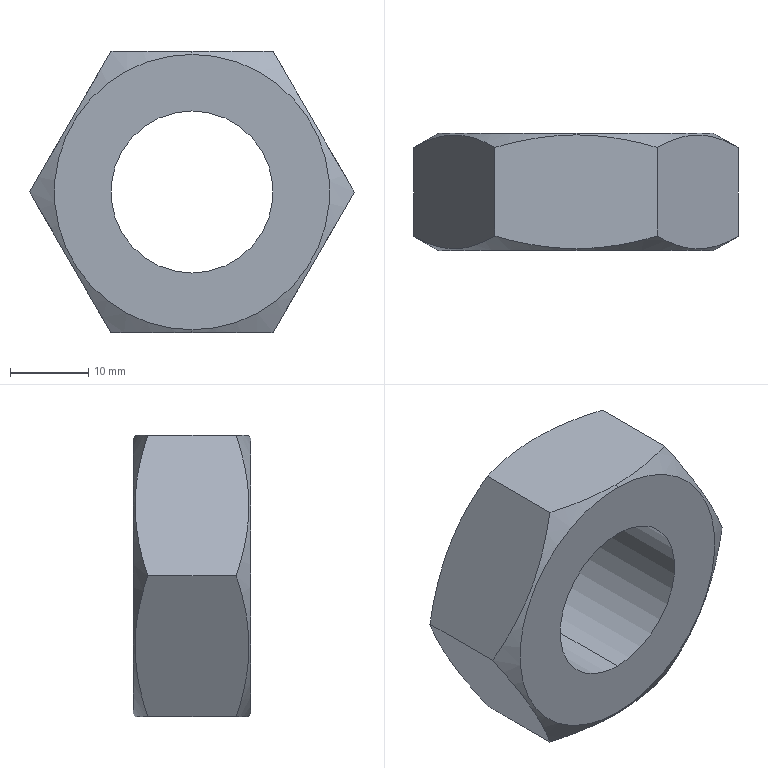Part | SolidWorks | features Extrusion 1, RevCut 1 | 1 solid | 14 faces | box 41.569 x 15 x 36.009 mm | volume 11607 mm3 | plane 8 | cone 4 | cylinder 2 | commonest cylinder face diameters 20.75 x2
STEP:
#1=CARTESIAN_POINT('',(0.,15.,-17.634));
#2=VERTEX_POINT('',#1);
#3=CARTESIAN_POINT('',(0.,15.,17.616));
#4=VERTEX_POINT('',#3);
#5=CARTESIAN_POINT('',(0.,15.,-0.008541));
#6=DIRECTION('',(0.,-1.,0.));
#7=DIRECTION('',(0.,0.,-1.));
#8=AXIS2_PLACEMENT_3D('',#5,#6,#7);
#9=CIRCLE('',#8,17.625);
#10=EDGE_CURVE('',#2,#4,#9,.T.);
#11=ORIENTED_EDGE('',*,*,#10,.T.);
#12=CARTESIAN_POINT('',(0.,14.779,18.));
#13=VERTEX_POINT('',#12);
#14=CARTESIAN_POINT('',(0.,14.786,17.987));
#15=DIRECTION('',(0.,-0.5,0.866));
#16=VECTOR('',#15,1000.);
#17=LINE('',#14,#16);
#18=EDGE_CURVE('',#4,#13,#17,.T.);
#19=ORIENTED_EDGE('',*,*,#18,.T.);
#20=CARTESIAN_POINT('',(10.4,13.172,17.996));
#21=VERTEX_POINT('',#20);
#22=CARTESIAN_POINT('',(10.4,13.172,17.996));
#23=CARTESIAN_POINT('',(8.698,13.662,17.996));
#24=CARTESIAN_POINT('',(6.985,14.067,17.997));
#25=CARTESIAN_POINT('',(3.522,14.626,17.999));
#26=CARTESIAN_POINT('',(1.772,14.779,17.999));
#27=CARTESIAN_POINT('',(0.,14.779,18.));
#28=B_SPLINE_CURVE_WITH_KNOTS('',3,(#22,#23,#24,#25,#26,#27),.UNSPECIFIED.,.F.,.F.,(4,2,4),(0.000000206,0.005261,0.01052),.UNSPECIFIED.);
#29=EDGE_CURVE('',#21,#13,#28,.T.);
#30=ORIENTED_EDGE('',*,*,#29,.F.);
#31=CARTESIAN_POINT('',(20.785,13.176,-0.008541));
#32=VERTEX_POINT('',#31);
#33=CARTESIAN_POINT('',(20.785,13.176,-0.008541));
#34=CARTESIAN_POINT('',(19.937,13.665,1.461));
#35=CARTESIAN_POINT('',(19.083,14.069,2.942));
#36=CARTESIAN_POINT('',(17.357,14.627,5.934));
#37=CARTESIAN_POINT('',(16.485,14.78,7.446));
#38=CARTESIAN_POINT('',(15.381,14.781,9.359));
#39=CARTESIAN_POINT('',(15.159,14.772,9.744));
#40=CARTESIAN_POINT('',(14.718,14.735,10.51));
#41=CARTESIAN_POINT('',(14.498,14.707,10.891));
#42=CARTESIAN_POINT('',(13.84,14.597,12.032));
#43=CARTESIAN_POINT('',(13.404,14.488,12.787));
#44=CARTESIAN_POINT('',(12.105,14.067,15.04));
#45=CARTESIAN_POINT('',(11.249,13.662,16.524));
#46=CARTESIAN_POINT('',(10.4,13.172,17.996));
#47=B_SPLINE_CURVE_WITH_KNOTS('',3,(#33,#34,#35,#36,#37,#38,#39,#40,#41,#42,#43,#44,#45,#46),.UNSPECIFIED.,.F.,.F.,(4,2,2,2,2,2,4),(0.000000238,0.005248,0.0105,0.01181,0.01312,0.01574,0.02099),.UNSPECIFIED.);
#48=EDGE_CURVE('',#32,#21,#47,.T.);
#49=ORIENTED_EDGE('',*,*,#48,.F.);
#50=CARTESIAN_POINT('',(10.385,13.18,-18.004));
#51=VERTEX_POINT('',#50);
#52=CARTESIAN_POINT('',(10.385,13.18,-18.004));
#53=CARTESIAN_POINT('',(11.234,13.67,-16.535));
#54=CARTESIAN_POINT('',(12.089,14.073,-15.055));
#55=CARTESIAN_POINT('',(13.818,14.632,-12.064));
#56=CARTESIAN_POINT('',(14.691,14.785,-10.553));
#57=CARTESIAN_POINT('',(15.796,14.786,-8.641));
#58=CARTESIAN_POINT('',(16.018,14.777,-8.256));
#59=CARTESIAN_POINT('',(16.461,14.74,-7.491));
#60=CARTESIAN_POINT('',(16.681,14.712,-7.11));
#61=CARTESIAN_POINT('',(17.34,14.602,-5.969));
#62=CARTESIAN_POINT('',(17.776,14.492,-5.214));
#63=CARTESIAN_POINT('',(19.077,14.072,-2.963));
#64=CARTESIAN_POINT('',(19.935,13.667,-1.479));
#65=CARTESIAN_POINT('',(20.785,13.176,-0.008541));
#66=B_SPLINE_CURVE_WITH_KNOTS('',3,(#52,#53,#54,#55,#56,#57,#58,#59,#60,#61,#62,#63,#64,#65),.UNSPECIFIED.,.F.,.F.,(4,2,2,2,2,2,4),(0.000000238,0.005248,0.0105,0.01181,0.01312,0.01574,0.02099),.UNSPECIFIED.);
#67=EDGE_CURVE('',#51,#32,#66,.T.);
#68=ORIENTED_EDGE('',*,*,#67,.F.);
#69=CARTESIAN_POINT('',(0.,14.788,-18.));
#70=VERTEX_POINT('',#69);
#71=CARTESIAN_POINT('',(0.,14.788,-18.));
#72=CARTESIAN_POINT('',(0.4407,14.788,-18.));
#73=CARTESIAN_POINT('',(0.8836,14.779,-18.));
#74=CARTESIAN_POINT('',(1.765,14.741,-18.001));
#75=CARTESIAN_POINT('',(2.204,14.713,-18.001));
#76=CARTESIAN_POINT('',(3.518,14.603,-18.001));
#77=CARTESIAN_POINT('',(4.388,14.494,-18.002));
#78=CARTESIAN_POINT('',(6.982,14.073,-18.003));
#79=CARTESIAN_POINT('',(8.69,13.669,-18.004));
#80=CARTESIAN_POINT('',(10.385,13.18,-18.004));
#81=B_SPLINE_CURVE_WITH_KNOTS('',3,(#71,#72,#73,#74,#75,#76,#77,#78,#79,#80),.UNSPECIFIED.,.F.,.F.,(4,2,2,2,4),(0.01052,0.01183,0.01314,0.01576,0.02099),.UNSPECIFIED.);
#82=EDGE_CURVE('',#70,#51,#81,.T.);
#83=ORIENTED_EDGE('',*,*,#82,.F.);
#84=CARTESIAN_POINT('',(0.,14.786,-18.004));
#85=DIRECTION('',(0.,-0.5,-0.866));
#86=VECTOR('',#85,1000.);
#87=LINE('',#84,#86);
#88=EDGE_CURVE('',#2,#70,#87,.T.);
#89=ORIENTED_EDGE('',*,*,#88,.F.);
#90=EDGE_LOOP('',(#11,#19,#30,#49,#68,#83,#89));
#91=FACE_OUTER_BOUND('',#90,.T.);
#92=CARTESIAN_POINT('',(0.,14.786,-0.008541));
#93=DIRECTION('',(0.,-1.,0.));
#94=DIRECTION('',(0.,0.,-1.));
#95=AXIS2_PLACEMENT_3D('',#92,#93,#94);
#96=CONICAL_SURFACE('',#95,17.996,1.047);
#97=ADVANCED_FACE('',(#91),#96,.T.);
#98=CARTESIAN_POINT('',(0.,0.,-17.634));
#99=VERTEX_POINT('',#98);
#100=CARTESIAN_POINT('',(0.,0.,17.616));
#101=VERTEX_POINT('',#100);
#102=CARTESIAN_POINT('',(0.,0.,-0.008541));
#103=DIRECTION('',(0.,-1.,0.));
#104=DIRECTION('',(0.,0.,-1.));
#105=AXIS2_PLACEMENT_3D('',#102,#103,#104);
#106=CIRCLE('',#105,17.625);
#107=EDGE_CURVE('',#99,#101,#106,.T.);
#108=ORIENTED_EDGE('',*,*,#107,.F.);
#109=CARTESIAN_POINT('',(0.,0.2116,-18.));
#110=VERTEX_POINT('',#109);
#111=CARTESIAN_POINT('',(0.,0.4553,-18.422));
#112=DIRECTION('',(0.,0.5,-0.866));
#113=VECTOR('',#112,1000.);
#114=LINE('',#111,#113);
#115=EDGE_CURVE('',#99,#110,#114,.T.);
#116=ORIENTED_EDGE('',*,*,#115,.T.);
#117=CARTESIAN_POINT('',(10.385,1.82,-18.004));
#118=VERTEX_POINT('',#117);
#119=CARTESIAN_POINT('',(10.385,1.82,-18.004));
#120=CARTESIAN_POINT('',(8.686,1.329,-18.004));
#121=CARTESIAN_POINT('',(6.975,0.9251,-18.003));
#122=CARTESIAN_POINT('',(3.517,0.3655,-18.001));
#123=CARTESIAN_POINT('',(1.769,0.212,-18.001));
#124=CARTESIAN_POINT('',(0.,0.2116,-18.));
#125=B_SPLINE_CURVE_WITH_KNOTS('',3,(#119,#120,#121,#122,#123,#124),.UNSPECIFIED.,.F.,.F.,(4,2,4),(0.000000206,0.005254,0.01051),.UNSPECIFIED.);
#126=EDGE_CURVE('',#118,#110,#125,.T.);
#127=ORIENTED_EDGE('',*,*,#126,.F.);
#128=CARTESIAN_POINT('',(20.785,1.824,-0.008541));
#129=VERTEX_POINT('',#128);
#130=CARTESIAN_POINT('',(20.785,1.824,-0.008541));
#131=CARTESIAN_POINT('',(19.936,1.334,-1.478));
#132=CARTESIAN_POINT('',(19.08,0.9299,-2.957));
#133=CARTESIAN_POINT('',(17.352,0.3698,-5.948));
#134=CARTESIAN_POINT('',(16.479,0.2156,-7.459));
#135=CARTESIAN_POINT('',(15.374,0.2137,-9.371));
#136=CARTESIAN_POINT('',(15.152,0.2227,-9.756));
#137=CARTESIAN_POINT('',(14.709,0.2595,-10.521));
#138=CARTESIAN_POINT('',(14.489,0.2872,-10.903));
#139=CARTESIAN_POINT('',(13.83,0.3968,-12.043));
#140=CARTESIAN_POINT('',(13.394,0.5054,-12.798));
#141=CARTESIAN_POINT('',(12.092,0.9251,-15.05));
#142=CARTESIAN_POINT('',(11.235,1.33,-16.533));
#143=CARTESIAN_POINT('',(10.385,1.82,-18.004));
#144=B_SPLINE_CURVE_WITH_KNOTS('',3,(#130,#131,#132,#133,#134,#135,#136,#137,#138,#139,#140,#141,#142,#143),.UNSPECIFIED.,.F.,.F.,(4,2,2,2,2,2,4),(0.000000238,0.005248,0.0105,0.01181,0.01312,0.01574,0.02099),.UNSPECIFIED.);
#145=EDGE_CURVE('',#129,#118,#144,.T.);
#146=ORIENTED_EDGE('',*,*,#145,.F.);
#147=CARTESIAN_POINT('',(10.4,1.828,17.996));
#148=VERTEX_POINT('',#147);
#149=CARTESIAN_POINT('',(10.4,1.828,17.996));
#150=CARTESIAN_POINT('',(11.247,1.338,16.526));
#151=CARTESIAN_POINT('',(12.101,0.9345,15.045));
#152=CARTESIAN_POINT('',(13.827,0.3746,12.053));
#153=CARTESIAN_POINT('',(14.699,0.2205,10.542));
#154=CARTESIAN_POINT('',(15.803,0.2186,8.628));
#155=CARTESIAN_POINT('',(16.025,0.2277,8.244));
#156=CARTESIAN_POINT('',(16.466,0.2644,7.478));
#157=CARTESIAN_POINT('',(16.686,0.2921,7.097));
#158=CARTESIAN_POINT('',(17.344,0.4016,5.956));
#159=CARTESIAN_POINT('',(17.78,0.5102,5.2));
#160=CARTESIAN_POINT('',(19.08,0.9297,2.947));
#161=CARTESIAN_POINT('',(19.936,1.334,1.463));
#162=CARTESIAN_POINT('',(20.785,1.824,-0.008541));
#163=B_SPLINE_CURVE_WITH_KNOTS('',3,(#149,#150,#151,#152,#153,#154,#155,#156,#157,#158,#159,#160,#161,#162),.UNSPECIFIED.,.F.,.F.,(4,2,2,2,2,2,4),(0.000000238,0.005248,0.0105,0.01181,0.01312,0.01574,0.02099),.UNSPECIFIED.);
#164=EDGE_CURVE('',#148,#129,#163,.T.);
#165=ORIENTED_EDGE('',*,*,#164,.F.);
#166=CARTESIAN_POINT('',(0.,0.2214,18.));
#167=VERTEX_POINT('',#166);
#168=CARTESIAN_POINT('',(0.,0.2214,18.));
#169=CARTESIAN_POINT('',(0.4413,0.2213,18.));
#170=CARTESIAN_POINT('',(0.8847,0.2307,18.));
#171=CARTESIAN_POINT('',(1.768,0.2679,17.999));
#172=CARTESIAN_POINT('',(2.208,0.2957,17.999));
#173=CARTESIAN_POINT('',(3.523,0.4058,17.999));
#174=CARTESIAN_POINT('',(4.394,0.5147,17.998));
#175=CARTESIAN_POINT('',(6.992,0.9346,17.997));
#176=CARTESIAN_POINT('',(8.703,1.339,17.996));
#177=CARTESIAN_POINT('',(10.4,1.828,17.996));
#178=B_SPLINE_CURVE_WITH_KNOTS('',3,(#168,#169,#170,#171,#172,#173,#174,#175,#176,#177),.UNSPECIFIED.,.F.,.F.,(4,2,2,2,4),(0.01051,0.01182,0.01313,0.01575,0.02099),.UNSPECIFIED.);
#179=EDGE_CURVE('',#167,#148,#178,.T.);
#180=ORIENTED_EDGE('',*,*,#179,.F.);
#181=CARTESIAN_POINT('',(0.,0.4553,18.405));
#182=DIRECTION('',(0.,0.5,0.866));
#183=VECTOR('',#182,1000.);
#184=LINE('',#181,#183);
#185=EDGE_CURVE('',#101,#167,#184,.T.);
#186=ORIENTED_EDGE('',*,*,#185,.F.);
#187=EDGE_LOOP('',(#108,#116,#127,#146,#165,#180,#186));
#188=FACE_OUTER_BOUND('',#187,.T.);
#189=CARTESIAN_POINT('',(0.,0.4553,-0.008541));
#190=DIRECTION('',(0.,1.,0.));
#191=DIRECTION('',(0.,0.,1.));
#192=AXIS2_PLACEMENT_3D('',#189,#190,#191);
#193=CONICAL_SURFACE('',#192,18.414,1.047);
#194=ADVANCED_FACE('',(#188),#193,.T.);
#195=CARTESIAN_POINT('',(0.,15.,-10.375));
#196=VERTEX_POINT('',#195);
#197=CARTESIAN_POINT('',(0.,15.,10.375));
#198=VERTEX_POINT('',#197);
#199=CARTESIAN_POINT('',(0.,15.,0.));
#200=DIRECTION('',(0.,1.,0.));
#201=DIRECTION('',(0.,0.,1.));
#202=AXIS2_PLACEMENT_3D('',#199,#200,#201);
#203=CIRCLE('',#202,10.375);
#204=EDGE_CURVE('',#196,#198,#203,.T.);
#205=ORIENTED_EDGE('',*,*,#204,.T.);
#206=CARTESIAN_POINT('',(0.,0.,10.375));
#207=VERTEX_POINT('',#206);
#208=CARTESIAN_POINT('',(0.,15.,10.375));
#209=DIRECTION('',(0.,-1.,0.));
#210=VECTOR('',#209,1000.);
#211=LINE('',#208,#210);
#212=EDGE_CURVE('',#198,#207,#211,.T.);
#213=ORIENTED_EDGE('',*,*,#212,.T.);
#214=CARTESIAN_POINT('',(0.,0.,-10.375));
#215=VERTEX_POINT('',#214);
#216=CARTESIAN_POINT('',(0.,0.,0.));
#217=DIRECTION('',(0.,1.,0.));
#218=DIRECTION('',(0.,0.,1.));
#219=AXIS2_PLACEMENT_3D('',#216,#217,#218);
#220=CIRCLE('',#219,10.375);
#221=EDGE_CURVE('',#215,#207,#220,.T.);
#222=ORIENTED_EDGE('',*,*,#221,.F.);
#223=CARTESIAN_POINT('',(0.,15.,-10.375));
#224=DIRECTION('',(0.,-1.,0.));
#225=VECTOR('',#224,1000.);
#226=LINE('',#223,#225);
#227=EDGE_CURVE('',#196,#215,#226,.T.);
#228=ORIENTED_EDGE('',*,*,#227,.F.);
#229=EDGE_LOOP('',(#205,#213,#222,#228));
#230=FACE_OUTER_BOUND('',#229,.T.);
#231=CARTESIAN_POINT('',(0.,15.,0.));
#232=DIRECTION('',(0.,-1.,0.));
#233=DIRECTION('',(0.,0.,-1.));
#234=AXIS2_PLACEMENT_3D('',#231,#232,#233);
#235=CYLINDRICAL_SURFACE('',#234,10.375);
#236=ADVANCED_FACE('',(#230),#235,.F.);
#237=ORIENTED_EDGE('',*,*,#204,.F.);
#238=CARTESIAN_POINT('',(0.,15.,0.));
#239=DIRECTION('',(0.,1.,0.));
#240=DIRECTION('',(0.,0.,1.));
#241=AXIS2_PLACEMENT_3D('',#238,#239,#240);
#242=CIRCLE('',#241,10.375);
#243=EDGE_CURVE('',#198,#196,#242,.T.);
#244=ORIENTED_EDGE('',*,*,#243,.F.);
#245=EDGE_LOOP('',(#237,#244));
#246=FACE_BOUND('',#245,.T.);
#247=ORIENTED_EDGE('',*,*,#10,.F.);
#248=CARTESIAN_POINT('',(0.,15.,-0.008541));
#249=DIRECTION('',(0.,-1.,0.));
#250=DIRECTION('',(0.,0.,-1.));
#251=AXIS2_PLACEMENT_3D('',#248,#249,#250);
#252=CIRCLE('',#251,17.625);
#253=EDGE_CURVE('',#4,#2,#252,.T.);
#254=ORIENTED_EDGE('',*,*,#253,.F.);
#255=EDGE_LOOP('',(#247,#254));
#256=FACE_OUTER_BOUND('',#255,.T.);
#257=CARTESIAN_POINT('',(0.,15.,0.));
#258=DIRECTION('',(0.,1.,0.));
#259=DIRECTION('',(0.,0.,1.));
#260=AXIS2_PLACEMENT_3D('',#257,#258,#259);
#261=PLANE('',#260);
#262=ADVANCED_FACE('',(#246,#256),#261,.T.);
#263=ORIENTED_EDGE('',*,*,#221,.T.);
#264=CARTESIAN_POINT('',(0.,0.,0.));
#265=DIRECTION('',(0.,1.,0.));
#266=DIRECTION('',(0.,0.,1.));
#267=AXIS2_PLACEMENT_3D('',#264,#265,#266);
#268=CIRCLE('',#267,10.375);
#269=EDGE_CURVE('',#207,#215,#268,.T.);
#270=ORIENTED_EDGE('',*,*,#269,.T.);
#271=EDGE_LOOP('',(#263,#270));
#272=FACE_BOUND('',#271,.T.);
#273=CARTESIAN_POINT('',(0.,0.,-0.008541));
#274=DIRECTION('',(0.,-1.,0.));
#275=DIRECTION('',(0.,0.,-1.));
#276=AXIS2_PLACEMENT_3D('',#273,#274,#275);
#277=CIRCLE('',#276,17.625);
#278=EDGE_CURVE('',#101,#99,#277,.T.);
#279=ORIENTED_EDGE('',*,*,#278,.T.);
#280=ORIENTED_EDGE('',*,*,#107,.T.);
#281=EDGE_LOOP('',(#279,#280));
#282=FACE_OUTER_BOUND('',#281,.T.);
#283=CARTESIAN_POINT('',(0.,0.,0.));
#284=DIRECTION('',(0.,1.,0.));
#285=DIRECTION('',(0.,0.,1.));
#286=AXIS2_PLACEMENT_3D('',#283,#284,#285);
#287=PLANE('',#286);
#288=ADVANCED_FACE('',(#272,#282),#287,.F.);
#289=ORIENTED_EDGE('',*,*,#212,.F.);
#290=ORIENTED_EDGE('',*,*,#243,.T.);
#291=ORIENTED_EDGE('',*,*,#227,.T.);
#292=ORIENTED_EDGE('',*,*,#269,.F.);
#293=EDGE_LOOP('',(#289,#290,#291,#292));
#294=FACE_OUTER_BOUND('',#293,.T.);
#295=CARTESIAN_POINT('',(0.,15.,0.));
#296=DIRECTION('',(0.,-1.,0.));
#297=DIRECTION('',(0.,0.,-1.));
#298=AXIS2_PLACEMENT_3D('',#295,#296,#297);
#299=CYLINDRICAL_SURFACE('',#298,10.375);
#300=ADVANCED_FACE('',(#294),#299,.F.);
#301=ORIENTED_EDGE('',*,*,#115,.F.);
#302=ORIENTED_EDGE('',*,*,#278,.F.);
#303=ORIENTED_EDGE('',*,*,#185,.T.);
#304=CARTESIAN_POINT('',(-10.385,1.828,18.004));
#305=VERTEX_POINT('',#304);
#306=CARTESIAN_POINT('',(-10.385,1.828,18.004));
#307=CARTESIAN_POINT('',(-8.686,1.338,18.004));
#308=CARTESIAN_POINT('',(-6.975,0.9343,18.003));
#309=CARTESIAN_POINT('',(-3.516,0.3752,18.001));
#310=CARTESIAN_POINT('',(-1.769,0.2219,18.001));
#311=CARTESIAN_POINT('',(0.,0.2214,18.));
#312=B_SPLINE_CURVE_WITH_KNOTS('',3,(#306,#307,#308,#309,#310,#311),.UNSPECIFIED.,.F.,.F.,(4,2,4),(0.000000206,0.005254,0.01051),.UNSPECIFIED.);
#313=EDGE_CURVE('',#305,#167,#312,.T.);
#314=ORIENTED_EDGE('',*,*,#313,.F.);
#315=CARTESIAN_POINT('',(-20.785,1.824,0.008541));
#316=VERTEX_POINT('',#315);
#317=CARTESIAN_POINT('',(-20.785,1.824,0.008541));
#318=CARTESIAN_POINT('',(-19.936,1.335,1.478));
#319=CARTESIAN_POINT('',(-19.08,0.9314,2.958));
#320=CARTESIAN_POINT('',(-17.352,0.3729,5.948));
#321=CARTESIAN_POINT('',(-16.479,0.2197,7.459));
#322=CARTESIAN_POINT('',(-15.374,0.2188,9.372));
#323=CARTESIAN_POINT('',(-15.151,0.2281,9.756));
#324=CARTESIAN_POINT('',(-14.709,0.2653,10.522));
#325=CARTESIAN_POINT('',(-14.489,0.2931,10.903));
#326=CARTESIAN_POINT('',(-13.83,0.4033,12.043));
#327=CARTESIAN_POINT('',(-13.393,0.5123,12.798));
#328=CARTESIAN_POINT('',(-12.092,0.9329,15.05));
#329=CARTESIAN_POINT('',(-11.235,1.338,16.533));
#330=CARTESIAN_POINT('',(-10.385,1.828,18.004));
#331=B_SPLINE_CURVE_WITH_KNOTS('',3,(#317,#318,#319,#320,#321,#322,#323,#324,#325,#326,#327,#328,#329,#330),.UNSPECIFIED.,.F.,.F.,(4,2,2,2,2,2,4),(0.000000238,0.005248,0.0105,0.01181,0.01312,0.01574,0.02099),.UNSPECIFIED.);
#332=EDGE_CURVE('',#316,#305,#331,.T.);
#333=ORIENTED_EDGE('',*,*,#332,.F.);
#334=CARTESIAN_POINT('',(-10.4,1.82,-17.996));
#335=VERTEX_POINT('',#334);
#336=CARTESIAN_POINT('',(-10.4,1.82,-17.996));
#337=CARTESIAN_POINT('',(-11.248,1.33,-16.526));
#338=CARTESIAN_POINT('',(-12.102,0.9267,-15.045));
#339=CARTESIAN_POINT('',(-13.827,0.3681,-12.053));
#340=CARTESIAN_POINT('',(-14.699,0.2147,-10.541));
#341=CARTESIAN_POINT('',(-15.803,0.2139,-8.628));
#342=CARTESIAN_POINT('',(-16.025,0.2232,-8.243));
#343=CARTESIAN_POINT('',(-16.467,0.2604,-7.477));
#344=CARTESIAN_POINT('',(-16.687,0.2883,-7.096));
#345=CARTESIAN_POINT('',(-17.345,0.3985,-5.955));
#346=CARTESIAN_POINT('',(-17.78,0.5075,-5.2));
#347=CARTESIAN_POINT('',(-19.08,0.9283,-2.947));
#348=CARTESIAN_POINT('',(-19.936,1.333,-1.463));
#349=CARTESIAN_POINT('',(-20.785,1.824,0.008541));
#350=B_SPLINE_CURVE_WITH_KNOTS('',3,(#336,#337,#338,#339,#340,#341,#342,#343,#344,#345,#346,#347,#348,#349),.UNSPECIFIED.,.F.,.F.,(4,2,2,2,2,2,4),(0.000000238,0.005248,0.0105,0.01181,0.01312,0.01574,0.02099),.UNSPECIFIED.);
#351=EDGE_CURVE('',#335,#316,#350,.T.);
#352=ORIENTED_EDGE('',*,*,#351,.F.);
#353=CARTESIAN_POINT('',(0.,0.2116,-18.));
#354=CARTESIAN_POINT('',(-0.4413,0.2115,-18.));
#355=CARTESIAN_POINT('',(-0.8848,0.2208,-18.));
#356=CARTESIAN_POINT('',(-1.768,0.2581,-17.999));
#357=CARTESIAN_POINT('',(-2.208,0.286,-17.999));
#358=CARTESIAN_POINT('',(-3.523,0.3962,-17.999));
#359=CARTESIAN_POINT('',(-4.394,0.5051,-17.998));
#360=CARTESIAN_POINT('',(-6.992,0.9254,-17.997));
#361=CARTESIAN_POINT('',(-8.703,1.33,-17.996));
#362=CARTESIAN_POINT('',(-10.4,1.82,-17.996));
#363=B_SPLINE_CURVE_WITH_KNOTS('',3,(#353,#354,#355,#356,#357,#358,#359,#360,#361,#362),.UNSPECIFIED.,.F.,.F.,(4,2,2,2,4),(0.01051,0.01182,0.01313,0.01575,0.02099),.UNSPECIFIED.);
#364=EDGE_CURVE('',#110,#335,#363,.T.);
#365=ORIENTED_EDGE('',*,*,#364,.F.);
#366=EDGE_LOOP('',(#301,#302,#303,#314,#333,#352,#365));
#367=FACE_OUTER_BOUND('',#366,.T.);
#368=CARTESIAN_POINT('',(0.,0.4553,-0.008541));
#369=DIRECTION('',(0.,1.,0.));
#370=DIRECTION('',(0.,0.,1.));
#371=AXIS2_PLACEMENT_3D('',#368,#369,#370);
#372=CONICAL_SURFACE('',#371,18.414,1.047);
#373=ADVANCED_FACE('',(#367),#372,.T.);
#374=ORIENTED_EDGE('',*,*,#18,.F.);
#375=ORIENTED_EDGE('',*,*,#253,.T.);
#376=ORIENTED_EDGE('',*,*,#88,.T.);
#377=CARTESIAN_POINT('',(-10.4,13.18,-17.996));
#378=VERTEX_POINT('',#377);
#379=CARTESIAN_POINT('',(-10.4,13.18,-17.996));
#380=CARTESIAN_POINT('',(-8.699,13.671,-17.996));
#381=CARTESIAN_POINT('',(-6.985,14.076,-17.997));
#382=CARTESIAN_POINT('',(-3.522,14.636,-17.999));
#383=CARTESIAN_POINT('',(-1.772,14.789,-17.999));
#384=CARTESIAN_POINT('',(0.,14.788,-18.));
#385=B_SPLINE_CURVE_WITH_KNOTS('',3,(#379,#380,#381,#382,#383,#384),.UNSPECIFIED.,.F.,.F.,(4,2,4),(0.000000206,0.005262,0.01052),.UNSPECIFIED.);
#386=EDGE_CURVE('',#378,#70,#385,.T.);
#387=ORIENTED_EDGE('',*,*,#386,.F.);
#388=CARTESIAN_POINT('',(-20.785,13.176,0.008541));
#389=VERTEX_POINT('',#388);
#390=CARTESIAN_POINT('',(-20.785,13.176,0.008541));
#391=CARTESIAN_POINT('',(-19.937,13.666,-1.461));
#392=CARTESIAN_POINT('',(-19.083,14.07,-2.942));
#393=CARTESIAN_POINT('',(-17.357,14.63,-5.934));
#394=CARTESIAN_POINT('',(-16.485,14.784,-7.445));
#395=CARTESIAN_POINT('',(-15.381,14.786,-9.359));
#396=CARTESIAN_POINT('',(-15.16,14.777,-9.743));
#397=CARTESIAN_POINT('',(-14.718,14.74,-10.509));
#398=CARTESIAN_POINT('',(-14.498,14.713,-10.891));
#399=CARTESIAN_POINT('',(-13.84,14.603,-12.032));
#400=CARTESIAN_POINT('',(-13.404,14.495,-12.787));
#401=CARTESIAN_POINT('',(-12.105,14.075,-15.04));
#402=CARTESIAN_POINT('',(-11.249,13.67,-16.524));
#403=CARTESIAN_POINT('',(-10.4,13.18,-17.996));
#404=B_SPLINE_CURVE_WITH_KNOTS('',3,(#390,#391,#392,#393,#394,#395,#396,#397,#398,#399,#400,#401,#402,#403),.UNSPECIFIED.,.F.,.F.,(4,2,2,2,2,2,4),(0.000000238,0.005248,0.0105,0.01181,0.01312,0.01574,0.02099),.UNSPECIFIED.);
#405=EDGE_CURVE('',#389,#378,#404,.T.);
#406=ORIENTED_EDGE('',*,*,#405,.F.);
#407=CARTESIAN_POINT('',(-10.385,13.172,18.004));
#408=VERTEX_POINT('',#407);
#409=CARTESIAN_POINT('',(-10.385,13.172,18.004));
#410=CARTESIAN_POINT('',(-11.234,13.662,16.535));
#411=CARTESIAN_POINT('',(-12.089,14.065,15.055));
#412=CARTESIAN_POINT('',(-13.817,14.625,12.065));
#413=CARTESIAN_POINT('',(-14.691,14.779,10.554));
#414=CARTESIAN_POINT('',(-15.796,14.781,8.641));
#415=CARTESIAN_POINT('',(-16.018,14.772,8.257));
#416=CARTESIAN_POINT('',(-16.46,14.736,7.492));
#417=CARTESIAN_POINT('',(-16.681,14.708,7.11));
#418=CARTESIAN_POINT('',(-17.34,14.598,5.97));
#419=CARTESIAN_POINT('',(-17.776,14.49,5.215));
#420=CARTESIAN_POINT('',(-19.077,14.07,2.963));
#421=CARTESIAN_POINT('',(-19.934,13.666,1.48));
#422=CARTESIAN_POINT('',(-20.785,13.176,0.008541));
#423=B_SPLINE_CURVE_WITH_KNOTS('',3,(#409,#410,#411,#412,#413,#414,#415,#416,#417,#418,#419,#420,#421,#422),.UNSPECIFIED.,.F.,.F.,(4,2,2,2,2,2,4),(0.000000238,0.005248,0.0105,0.01181,0.01312,0.01574,0.02099),.UNSPECIFIED.);
#424=EDGE_CURVE('',#408,#389,#423,.T.);
#425=ORIENTED_EDGE('',*,*,#424,.F.);
#426=CARTESIAN_POINT('',(0.,14.779,18.));
#427=CARTESIAN_POINT('',(-0.4407,14.778,18.));
#428=CARTESIAN_POINT('',(-0.8835,14.769,18.));
#429=CARTESIAN_POINT('',(-1.765,14.731,18.001));
#430=CARTESIAN_POINT('',(-2.204,14.703,18.001));
#431=CARTESIAN_POINT('',(-3.518,14.593,18.001));
#432=CARTESIAN_POINT('',(-4.388,14.484,18.002));
#433=CARTESIAN_POINT('',(-6.982,14.064,18.003));
#434=CARTESIAN_POINT('',(-8.69,13.661,18.004));
#435=CARTESIAN_POINT('',(-10.385,13.172,18.004));
#436=B_SPLINE_CURVE_WITH_KNOTS('',3,(#426,#427,#428,#429,#430,#431,#432,#433,#434,#435),.UNSPECIFIED.,.F.,.F.,(4,2,2,2,4),(0.01052,0.01183,0.01314,0.01576,0.02099),.UNSPECIFIED.);
#437=EDGE_CURVE('',#13,#408,#436,.T.);
#438=ORIENTED_EDGE('',*,*,#437,.F.);
#439=EDGE_LOOP('',(#374,#375,#376,#387,#406,#425,#438));
#440=FACE_OUTER_BOUND('',#439,.T.);
#441=CARTESIAN_POINT('',(0.,14.786,-0.008541));
#442=DIRECTION('',(0.,-1.,0.));
#443=DIRECTION('',(0.,0.,-1.));
#444=AXIS2_PLACEMENT_3D('',#441,#442,#443);
#445=CONICAL_SURFACE('',#444,17.996,1.047);
#446=ADVANCED_FACE('',(#440),#445,.T.);
#447=CARTESIAN_POINT('',(20.785,15.,-0.008541));
#448=DIRECTION('',(0.,-1.,0.));
#449=VECTOR('',#448,1000.);
#450=LINE('',#447,#449);
#451=EDGE_CURVE('',#32,#129,#450,.T.);
#452=ORIENTED_EDGE('',*,*,#451,.F.);
#453=ORIENTED_EDGE('',*,*,#48,.T.);
#454=CARTESIAN_POINT('',(10.4,15.,17.996));
#455=DIRECTION('',(0.,-1.,0.));
#456=VECTOR('',#455,1000.);
#457=LINE('',#454,#456);
#458=EDGE_CURVE('',#21,#148,#457,.T.);
#459=ORIENTED_EDGE('',*,*,#458,.T.);
#460=ORIENTED_EDGE('',*,*,#164,.T.);
#461=EDGE_LOOP('',(#452,#453,#459,#460));
#462=FACE_OUTER_BOUND('',#461,.T.);
#463=CARTESIAN_POINT('',(10.4,15.,17.996));
#464=DIRECTION('',(-0.8662,0.,-0.4996));
#465=DIRECTION('',(-0.4996,0.,0.8662));
#466=AXIS2_PLACEMENT_3D('',#463,#464,#465);
#467=PLANE('',#466);
#468=ADVANCED_FACE('',(#462),#467,.F.);
#469=ORIENTED_EDGE('',*,*,#458,.F.);
#470=ORIENTED_EDGE('',*,*,#29,.T.);
#471=ORIENTED_EDGE('',*,*,#437,.T.);
#472=CARTESIAN_POINT('',(-10.385,15.,18.004));
#473=DIRECTION('',(0.,-1.,0.));
#474=VECTOR('',#473,1000.);
#475=LINE('',#472,#474);
#476=EDGE_CURVE('',#408,#305,#475,.T.);
#477=ORIENTED_EDGE('',*,*,#476,.T.);
#478=ORIENTED_EDGE('',*,*,#313,.T.);
#479=ORIENTED_EDGE('',*,*,#179,.T.);
#480=EDGE_LOOP('',(#469,#470,#471,#477,#478,#479));
#481=FACE_OUTER_BOUND('',#480,.T.);
#482=CARTESIAN_POINT('',(-10.385,15.,18.004));
#483=DIRECTION('',(-0.0004109,0.,-1.));
#484=DIRECTION('',(-1.,0.,0.0004109));
#485=AXIS2_PLACEMENT_3D('',#482,#483,#484);
#486=PLANE('',#485);
#487=ADVANCED_FACE('',(#481),#486,.F.);
#488=ORIENTED_EDGE('',*,*,#476,.F.);
#489=ORIENTED_EDGE('',*,*,#424,.T.);
#490=CARTESIAN_POINT('',(-20.785,15.,0.008541));
#491=DIRECTION('',(0.,-1.,0.));
#492=VECTOR('',#491,1000.);
#493=LINE('',#490,#492);
#494=EDGE_CURVE('',#389,#316,#493,.T.);
#495=ORIENTED_EDGE('',*,*,#494,.T.);
#496=ORIENTED_EDGE('',*,*,#332,.T.);
#497=EDGE_LOOP('',(#488,#489,#495,#496));
#498=FACE_OUTER_BOUND('',#497,.T.);
#499=CARTESIAN_POINT('',(-20.785,15.,0.008541));
#500=DIRECTION('',(0.8658,0.,-0.5004));
#501=DIRECTION('',(-0.5004,0.,-0.8658));
#502=AXIS2_PLACEMENT_3D('',#499,#500,#501);
#503=PLANE('',#502);
#504=ADVANCED_FACE('',(#498),#503,.F.);
#505=ORIENTED_EDGE('',*,*,#494,.F.);
#506=ORIENTED_EDGE('',*,*,#405,.T.);
#507=CARTESIAN_POINT('',(-10.4,15.,-17.996));
#508=DIRECTION('',(0.,-1.,0.));
#509=VECTOR('',#508,1000.);
#510=LINE('',#507,#509);
#511=EDGE_CURVE('',#378,#335,#510,.T.);
#512=ORIENTED_EDGE('',*,*,#511,.T.);
#513=ORIENTED_EDGE('',*,*,#351,.T.);
#514=EDGE_LOOP('',(#505,#506,#512,#513));
#515=FACE_OUTER_BOUND('',#514,.T.);
#516=CARTESIAN_POINT('',(-10.4,15.,-17.996));
#517=DIRECTION('',(0.8662,0.,0.4996));
#518=DIRECTION('',(0.4996,0.,-0.8662));
#519=AXIS2_PLACEMENT_3D('',#516,#517,#518);
#520=PLANE('',#519);
#521=ADVANCED_FACE('',(#515),#520,.F.);
#522=ORIENTED_EDGE('',*,*,#511,.F.);
#523=ORIENTED_EDGE('',*,*,#386,.T.);
#524=ORIENTED_EDGE('',*,*,#82,.T.);
#525=CARTESIAN_POINT('',(10.385,15.,-18.004));
#526=DIRECTION('',(0.,-1.,0.));
#527=VECTOR('',#526,1000.);
#528=LINE('',#525,#527);
#529=EDGE_CURVE('',#51,#118,#528,.T.);
#530=ORIENTED_EDGE('',*,*,#529,.T.);
#531=ORIENTED_EDGE('',*,*,#126,.T.);
#532=ORIENTED_EDGE('',*,*,#364,.T.);
#533=EDGE_LOOP('',(#522,#523,#524,#530,#531,#532));
#534=FACE_OUTER_BOUND('',#533,.T.);
#535=CARTESIAN_POINT('',(10.385,15.,-18.004));
#536=DIRECTION('',(0.0004109,0.,1.));
#537=DIRECTION('',(1.,0.,-0.0004109));
#538=AXIS2_PLACEMENT_3D('',#535,#536,#537);
#539=PLANE('',#538);
#540=ADVANCED_FACE('',(#534),#539,.F.);
#541=ORIENTED_EDGE('',*,*,#529,.F.);
#542=ORIENTED_EDGE('',*,*,#67,.T.);
#543=ORIENTED_EDGE('',*,*,#451,.T.);
#544=ORIENTED_EDGE('',*,*,#145,.T.);
#545=EDGE_LOOP('',(#541,#542,#543,#544));
#546=FACE_OUTER_BOUND('',#545,.T.);
#547=CARTESIAN_POINT('',(20.785,15.,-0.008541));
#548=DIRECTION('',(-0.8658,0.,0.5004));
#549=DIRECTION('',(0.5004,0.,0.8658));
#550=AXIS2_PLACEMENT_3D('',#547,#548,#549);
#551=PLANE('',#550);
#552=ADVANCED_FACE('',(#546),#551,.F.);
#553=CLOSED_SHELL('',(#97,#194,#236,#262,#288,#300,#373,#446,#468,#487,#504,#521,#540,#552));
#554=MANIFOLD_SOLID_BREP('',#553);
#555=CARTESIAN_POINT('',(0.,0.,0.));
#556=DIRECTION('',(0.,0.,1.));
#557=DIRECTION('',(1.,0.,0.));
#558=AXIS2_PLACEMENT_3D('',#555,#556,#557);
#559=(LENGTH_UNIT()NAMED_UNIT(*)SI_UNIT(.MILLI.,.METRE.));
#560=UNCERTAINTY_MEASURE_WITH_UNIT(LENGTH_MEASURE(0.00001),#559,'','');
#561=(NAMED_UNIT(*)PLANE_ANGLE_UNIT()SI_UNIT($,.RADIAN.));
#562=(NAMED_UNIT(*)SI_UNIT($,.STERADIAN.)SOLID_ANGLE_UNIT());
#563=(GEOMETRIC_REPRESENTATION_CONTEXT(3)GLOBAL_UNCERTAINTY_ASSIGNED_CONTEXT((#560))GLOBAL_UNIT_ASSIGNED_CONTEXT((#559,#561,#562))REPRESENTATION_CONTEXT('',''));
#564=ADVANCED_BREP_SHAPE_REPRESENTATION('',(#554,#558),#563);